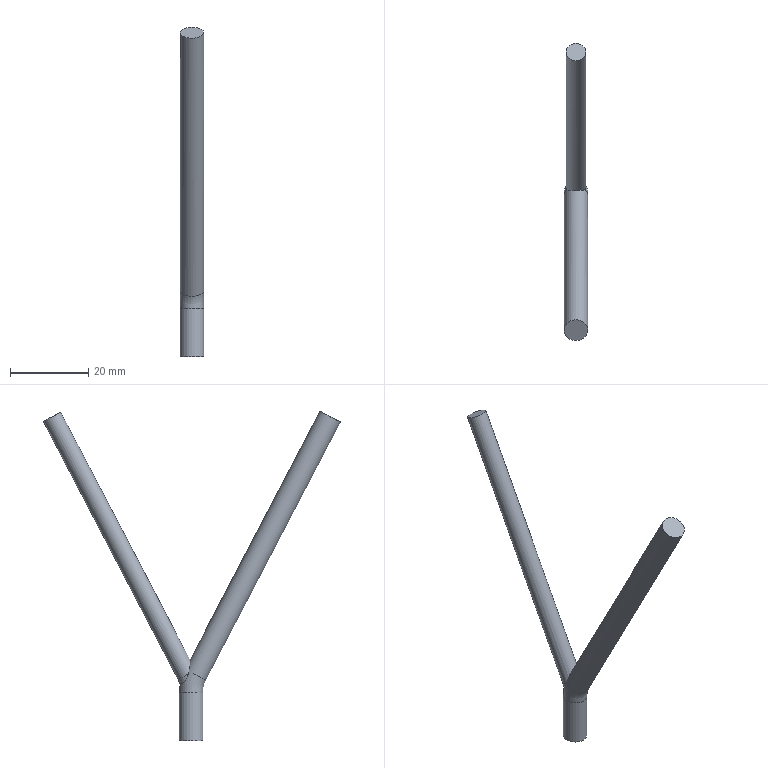Part | NX | features DATUM_CSYS 2, SWP104 2, SKETCH 1 | 1 solid | 8 faces | box 6 x 76.071 x 84.286 mm | volume 4037 mm3 | cylinder 3 | plane 3 | torus 2 | commonest cylinder face diameters 6 x2 5 x1
STEP:
#1=CARTESIAN_POINT('',(-2.322,0.5491,17.731));
#2=VERTEX_POINT('',#1);
#3=CARTESIAN_POINT('',(-2.447,0.6805,17.09));
#4=VERTEX_POINT('',#3);
#5=CARTESIAN_POINT('',(-2.322,0.5491,17.731));
#6=CARTESIAN_POINT('',(-2.375,0.5875,17.518));
#7=CARTESIAN_POINT('',(-2.417,0.6297,17.304));
#8=CARTESIAN_POINT('',(-2.447,0.6805,17.09));
#9=B_SPLINE_CURVE_WITH_KNOTS('',3,(#5,#6,#7,#8),.UNSPECIFIED.,.F.,.F.,(4,4),(0.0005335,0.0012),.UNSPECIFIED.);
#10=EDGE_CURVE('',#2,#4,#9,.T.);
#11=ORIENTED_EDGE('',*,*,#10,.F.);
#12=CARTESIAN_POINT('',(2.322,0.5491,17.731));
#13=VERTEX_POINT('',#12);
#14=CARTESIAN_POINT('',(-2.322,0.5491,17.731));
#15=CARTESIAN_POINT('',(-2.165,0.4351,18.366));
#16=CARTESIAN_POINT('',(-1.82,0.3577,19.285));
#17=CARTESIAN_POINT('',(-0.9777,0.2948,20.337));
#18=CARTESIAN_POINT('',(-0.007227,0.2757,20.765));
#19=CARTESIAN_POINT('',(0.9709,0.2945,20.343));
#20=CARTESIAN_POINT('',(1.809,0.3563,19.303));
#21=CARTESIAN_POINT('',(2.165,0.4349,18.367));
#22=CARTESIAN_POINT('',(2.322,0.5491,17.731));
#23=B_SPLINE_CURVE_WITH_KNOTS('',3,(#14,#15,#16,#17,#18,#19,#20,#21,#22),.UNSPECIFIED.,.F.,.F.,(4,1,1,1,1,1,4),(0.,0.00196,0.00294,0.003921,0.004901,0.005881,0.007841),.UNSPECIFIED.);
#24=EDGE_CURVE('',#2,#13,#23,.T.);
#25=ORIENTED_EDGE('',*,*,#24,.T.);
#26=CARTESIAN_POINT('',(2.447,0.6805,17.09));
#27=VERTEX_POINT('',#26);
#28=CARTESIAN_POINT('',(2.447,0.6805,17.09));
#29=CARTESIAN_POINT('',(2.417,0.6298,17.304));
#30=CARTESIAN_POINT('',(2.375,0.5875,17.518));
#31=CARTESIAN_POINT('',(2.322,0.5491,17.731));
#32=B_SPLINE_CURVE_WITH_KNOTS('',3,(#28,#29,#30,#31),.UNSPECIFIED.,.F.,.F.,(4,4),(0.001517,0.002182),.UNSPECIFIED.);
#33=EDGE_CURVE('',#27,#13,#32,.T.);
#34=ORIENTED_EDGE('',*,*,#33,.F.);
#35=CARTESIAN_POINT('',(0.,1.134,16.853));
#36=DIRECTION('',(0.,0.4626,0.8866));
#37=DIRECTION('',(0.,-0.8866,0.4626));
#38=AXIS2_PLACEMENT_3D('',#35,#36,#37);
#39=CIRCLE('',#38,2.5);
#40=EDGE_CURVE('',#27,#4,#39,.T.);
#41=ORIENTED_EDGE('',*,*,#40,.T.);
#42=EDGE_LOOP('',(#11,#25,#34,#41));
#43=FACE_BOUND('',#42,.T.);
#44=CARTESIAN_POINT('',(0.,33.381,84.055));
#45=VERTEX_POINT('',#44);
#46=CARTESIAN_POINT('',(0.,35.598,82.898));
#47=DIRECTION('',(0.,0.4626,0.8866));
#48=DIRECTION('',(0.,-0.8866,0.4626));
#49=AXIS2_PLACEMENT_3D('',#46,#47,#48);
#50=CIRCLE('',#49,2.5);
#51=EDGE_CURVE('',#45,#45,#50,.T.);
#52=ORIENTED_EDGE('',*,*,#51,.F.);
#53=EDGE_LOOP('',(#52));
#54=FACE_BOUND('',#53,.T.);
#55=CARTESIAN_POINT('',(0.,1.134,16.853));
#56=DIRECTION('',(0.,0.4626,0.8866));
#57=DIRECTION('',(0.,-0.8866,0.4626));
#58=AXIS2_PLACEMENT_3D('',#55,#56,#57);
#59=CYLINDRICAL_SURFACE('',#58,2.5);
#60=ADVANCED_FACE('',(#43,#54),#59,.T.);
#61=CARTESIAN_POINT('',(-2.447,0.6805,17.09));
#62=CARTESIAN_POINT('',(-2.503,0.7748,16.692));
#63=CARTESIAN_POINT('',(-2.543,1.028,15.878));
#64=CARTESIAN_POINT('',(-2.188,1.831,14.919));
#65=CARTESIAN_POINT('',(-1.252,2.624,14.476));
#66=CARTESIAN_POINT('',(-0.00002066,2.916,14.347));
#67=CARTESIAN_POINT('',(1.248,2.625,14.475));
#68=CARTESIAN_POINT('',(2.186,1.834,14.916));
#69=CARTESIAN_POINT('',(2.543,1.028,15.877));
#70=CARTESIAN_POINT('',(2.503,0.7757,16.689));
#71=CARTESIAN_POINT('',(2.447,0.6805,17.09));
#72=B_SPLINE_CURVE_WITH_KNOTS('',3,(#61,#62,#63,#64,#65,#66,#67,#68,#69,#70,#71),.UNSPECIFIED.,.F.,.F.,(4,1,1,1,1,1,1,1,4),(0.0009557,0.002192,0.003429,0.004665,0.005902,0.007138,0.008374,0.009611,0.01085),.UNSPECIFIED.);
#73=EDGE_CURVE('',#4,#27,#72,.T.);
#74=ORIENTED_EDGE('',*,*,#73,.F.);
#75=ORIENTED_EDGE('',*,*,#40,.F.);
#76=EDGE_LOOP('',(#74,#75));
#77=FACE_BOUND('',#76,.T.);
#78=CARTESIAN_POINT('',(0.,10.,12.227));
#79=DIRECTION('',(-1.,0.,0.));
#80=DIRECTION('',(0.,0.,1.));
#81=AXIS2_PLACEMENT_3D('',#78,#79,#80);
#82=TOROIDAL_SURFACE('',#81,10.,2.5);
#83=ADVANCED_FACE('',(#77),#82,.T.);
#84=ORIENTED_EDGE('',*,*,#51,.T.);
#85=EDGE_LOOP('',(#84));
#86=FACE_BOUND('',#85,.T.);
#87=CARTESIAN_POINT('',(0.,35.598,82.898));
#88=DIRECTION('',(0.,0.4626,0.8866));
#89=DIRECTION('',(0.,-0.8866,0.4626));
#90=AXIS2_PLACEMENT_3D('',#87,#88,#89);
#91=PLANE('',#90);
#92=ADVANCED_FACE('',(#86),#91,.T.);
#93=CARTESIAN_POINT('',(0.,3.,12.227));
#94=VERTEX_POINT('',#93);
#95=CARTESIAN_POINT('',(0.,0.,12.227));
#96=DIRECTION('',(0.,0.,-1.));
#97=DIRECTION('',(0.,1.,0.));
#98=AXIS2_PLACEMENT_3D('',#95,#96,#97);
#99=CIRCLE('',#98,3.);
#100=EDGE_CURVE('',#94,#94,#99,.T.);
#101=ORIENTED_EDGE('',*,*,#100,.T.);
#102=EDGE_LOOP('',(#101));
#103=FACE_BOUND('',#102,.T.);
#104=CARTESIAN_POINT('',(0.,3.,0.));
#105=VERTEX_POINT('',#104);
#106=CARTESIAN_POINT('',(0.,0.,0.));
#107=DIRECTION('',(0.,0.,-1.));
#108=DIRECTION('',(0.,1.,0.));
#109=AXIS2_PLACEMENT_3D('',#106,#107,#108);
#110=CIRCLE('',#109,3.);
#111=EDGE_CURVE('',#105,#105,#110,.T.);
#112=ORIENTED_EDGE('',*,*,#111,.F.);
#113=EDGE_LOOP('',(#112));
#114=FACE_BOUND('',#113,.T.);
#115=CARTESIAN_POINT('',(0.,0.,12.227));
#116=DIRECTION('',(0.,0.,-1.));
#117=DIRECTION('',(0.,1.,0.));
#118=AXIS2_PLACEMENT_3D('',#115,#116,#117);
#119=CYLINDRICAL_SURFACE('',#118,3.);
#120=ADVANCED_FACE('',(#103,#114),#119,.T.);
#121=CARTESIAN_POINT('',(0.,-1.134,16.853));
#122=DIRECTION('',(0.,0.4626,-0.8866));
#123=DIRECTION('',(0.,0.8866,0.4626));
#124=AXIS2_PLACEMENT_3D('',#121,#122,#123);
#125=CIRCLE('',#124,3.);
#126=EDGE_CURVE('',#13,#2,#125,.T.);
#127=ORIENTED_EDGE('',*,*,#126,.T.);
#128=ORIENTED_EDGE('',*,*,#10,.T.);
#129=ORIENTED_EDGE('',*,*,#73,.T.);
#130=ORIENTED_EDGE('',*,*,#33,.T.);
#131=EDGE_LOOP('',(#127,#128,#129,#130));
#132=FACE_BOUND('',#131,.T.);
#133=ORIENTED_EDGE('',*,*,#100,.F.);
#134=EDGE_LOOP('',(#133));
#135=FACE_BOUND('',#134,.T.);
#136=CARTESIAN_POINT('',(0.,-10.,12.227));
#137=DIRECTION('',(-1.,0.,0.));
#138=DIRECTION('',(0.,0.,1.));
#139=AXIS2_PLACEMENT_3D('',#136,#137,#138);
#140=TOROIDAL_SURFACE('',#139,10.,3.);
#141=ADVANCED_FACE('',(#132,#135),#140,.T.);
#142=ORIENTED_EDGE('',*,*,#24,.F.);
#143=ORIENTED_EDGE('',*,*,#126,.F.);
#144=EDGE_LOOP('',(#142,#143));
#145=FACE_BOUND('',#144,.T.);
#146=CARTESIAN_POINT('',(0.,-32.938,84.286));
#147=VERTEX_POINT('',#146);
#148=CARTESIAN_POINT('',(0.,-35.598,82.898));
#149=DIRECTION('',(0.,0.4626,-0.8866));
#150=DIRECTION('',(0.,0.8866,0.4626));
#151=AXIS2_PLACEMENT_3D('',#148,#149,#150);
#152=CIRCLE('',#151,3.);
#153=EDGE_CURVE('',#147,#147,#152,.T.);
#154=ORIENTED_EDGE('',*,*,#153,.T.);
#155=EDGE_LOOP('',(#154));
#156=FACE_BOUND('',#155,.T.);
#157=CARTESIAN_POINT('',(0.,-1.134,16.853));
#158=DIRECTION('',(0.,-0.4626,0.8866));
#159=DIRECTION('',(0.,-0.8866,-0.4626));
#160=AXIS2_PLACEMENT_3D('',#157,#158,#159);
#161=CYLINDRICAL_SURFACE('',#160,3.);
#162=ADVANCED_FACE('',(#145,#156),#161,.T.);
#163=ORIENTED_EDGE('',*,*,#153,.F.);
#164=EDGE_LOOP('',(#163));
#165=FACE_BOUND('',#164,.T.);
#166=CARTESIAN_POINT('',(0.,-35.598,82.898));
#167=DIRECTION('',(0.,0.4626,-0.8866));
#168=DIRECTION('',(0.,0.8866,0.4626));
#169=AXIS2_PLACEMENT_3D('',#166,#167,#168);
#170=PLANE('',#169);
#171=ADVANCED_FACE('',(#165),#170,.F.);
#172=ORIENTED_EDGE('',*,*,#111,.T.);
#173=EDGE_LOOP('',(#172));
#174=FACE_BOUND('',#173,.T.);
#175=CARTESIAN_POINT('',(0.,0.,0.));
#176=DIRECTION('',(0.,0.,1.));
#177=DIRECTION('',(0.,-1.,0.));
#178=AXIS2_PLACEMENT_3D('',#175,#176,#177);
#179=PLANE('',#178);
#180=ADVANCED_FACE('',(#174),#179,.F.);
#181=CLOSED_SHELL('',(#60,#83,#92,#120,#141,#162,#171,#180));
#182=MANIFOLD_SOLID_BREP('',#181);
#183=(LENGTH_UNIT()NAMED_UNIT(*)SI_UNIT(.MILLI.,.METRE.));
#184=UNCERTAINTY_MEASURE_WITH_UNIT(LENGTH_MEASURE(0.0508),#183,'','');
#185=(NAMED_UNIT(*)PLANE_ANGLE_UNIT()SI_UNIT($,.RADIAN.));
#186=(NAMED_UNIT(*)SI_UNIT($,.STERADIAN.)SOLID_ANGLE_UNIT());
#187=(GEOMETRIC_REPRESENTATION_CONTEXT(3)GLOBAL_UNCERTAINTY_ASSIGNED_CONTEXT((#184))GLOBAL_UNIT_ASSIGNED_CONTEXT((#183,#185,#186))REPRESENTATION_CONTEXT('',''));
#188=ADVANCED_BREP_SHAPE_REPRESENTATION('',(#182),#187);